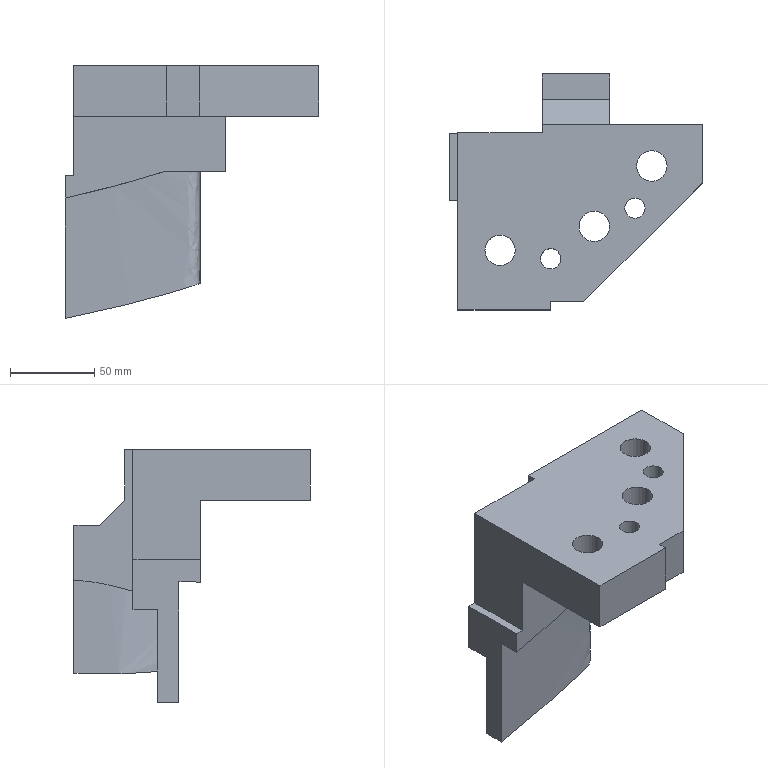Part | NX | features solid 2 | 1 solid | 36 faces | box 150.075 x 140 x 149.917 mm | volume 640785 mm3 | plane 21 | cylinder 8 | spline 7 | commonest cylinder face diameters 18 x3 26 x3 12 x2